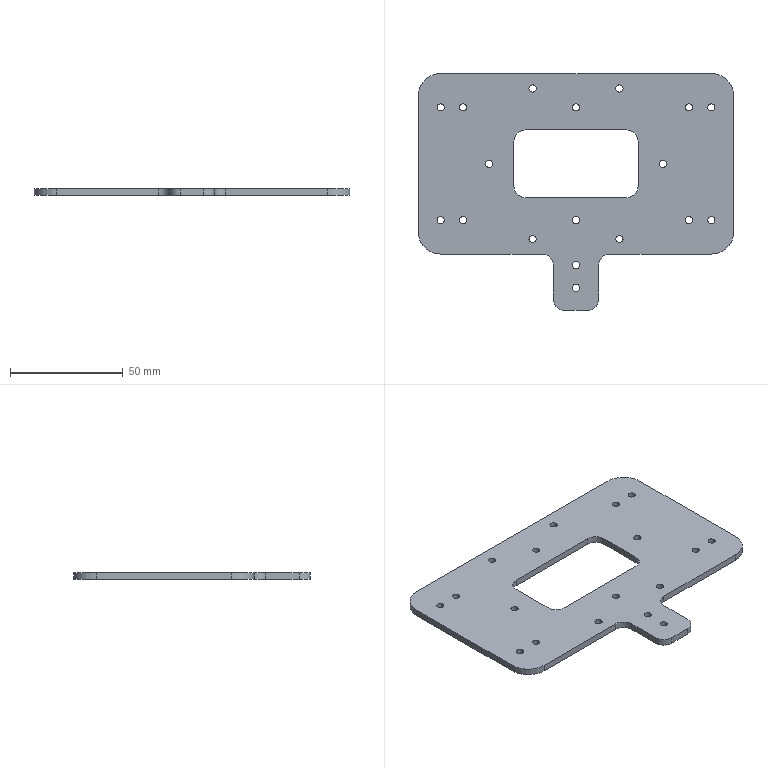Part | SolidWorks | features BaseBody 1 | 1 solid | 62 faces | box 140 x 105 x 3 mm | volume 29523 mm3 | cylinder 48 | plane 14 | commonest cylinder face diameters 3.2 x36 10 x8 20 x4